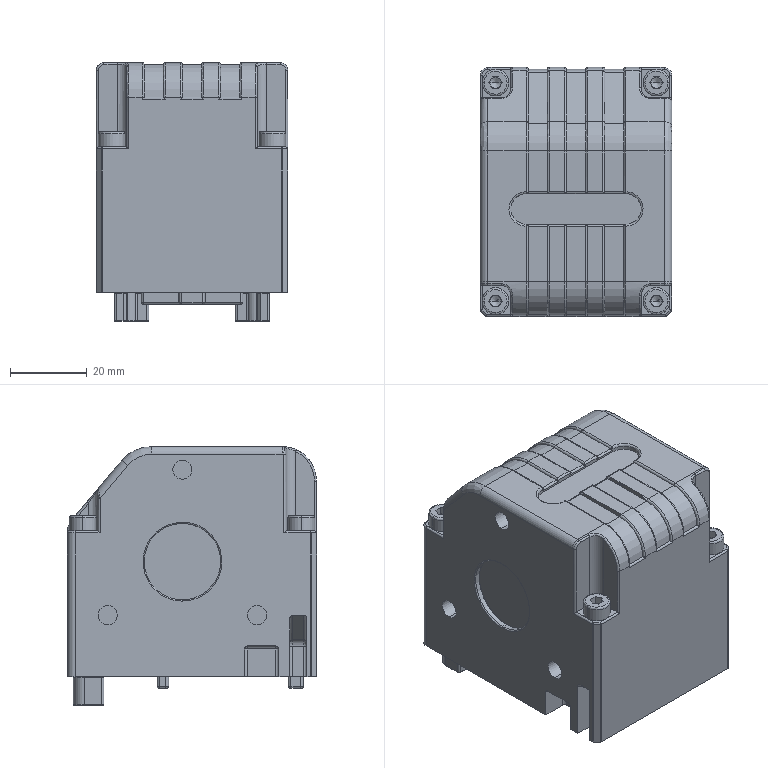Part | STEP file | Copy of K50-001A^K50A-1H20-S(formula driven)-L300-motor left- | 7 solids | 708 faces | box 50 x 65 x 67.5 mm | volume 172642 mm3 | cylinder 291 | plane 205 | spline 188 | cone 24 | commonest cylinder face diameters 1 x85 5 x38 0.4 x24 4 x20 1.6 x18 0.6 x12